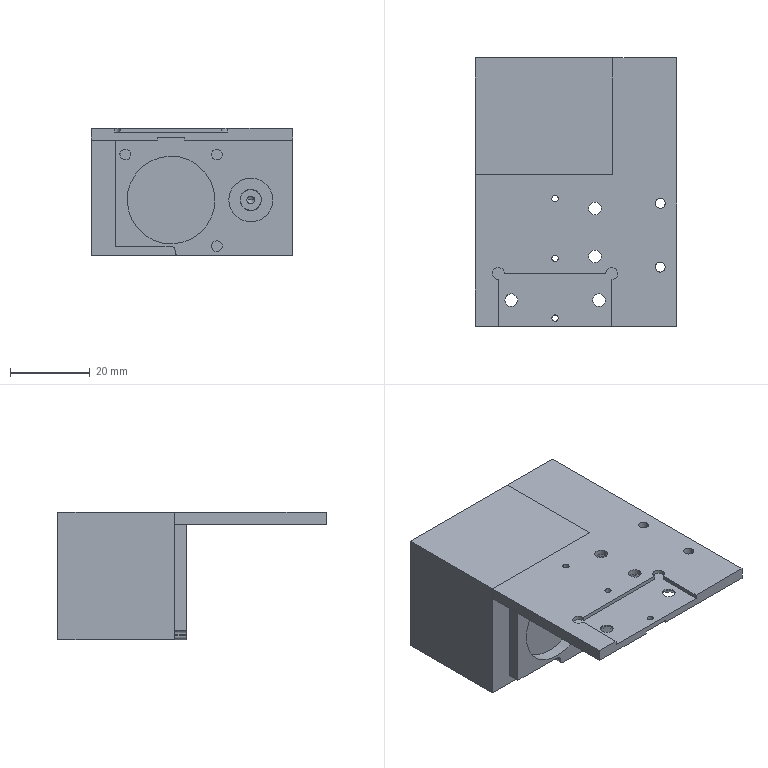NC program | NX | posted with a generic post | part box 50.5 x 67.3 x 32 mm
Whole program:
N10 G17 G21 G94 G90
(ZLEVEL_PROFILE , TOOL : D10)
N12 T10 M6
N14 G54
N16 G17 G0 G90 X35.272 Y-32.059 B0. C0. S9500 M3
N18 G43 Z30. H10
N20 Z-14.5
N22 G94 G1 Z-16. F1500.
N24 X34.516 Y-30.75
N26 G3 X33.65 Y-30.25 R1.
N28 G1 X-33.65
N30 G2 X-38.65 Y-25.25 R5.
N32 G1 Y25.25
N34 G2 X-33.65 Y30.25 R5.
N36 G1 X33.65
N38 G2 X38.65 Y25.25 R5.
N40 G1 Y-25.25
N42 G2 X33.65 Y-30.25 R5.
N44 G3 X32.784 Y-30.75 R1.
N46 G1 X31.918 Y-32.25
N48 Z-14.5
N50 G0 Z30.
N52 X35.272 Y-32.059
N54 Z-30.5
N56 G1 Z-32.
N58 X34.516 Y-30.75
N60 G3 X33.65 Y-30.25 R1.
N62 G1 X-33.65
N64 G2 X-38.65 Y-25.25 R5.
N66 G1 Y25.25
N68 G2 X-33.65 Y30.25 R5.
N70 G1 X33.65
N72 G2 X38.65 Y25.25 R5.
N74 G1 Y-25.25
N76 G2 X33.65 Y-30.25 R5.
N78 G3 X32.784 Y-30.75 R1.
N80 G1 X31.918 Y-32.25
N82 Z-30.5
N84 G0 Z30.
N86 M5
(FLOOR_WALL_1_COPY_1 , TOOL : D4)
N88 T04 M6
N90 G54
N92 G17 G0 G90 X36.65 Y-4.442 B0. C0. S9500 M3
N94 G43 Z30. H4
N96 Z-0.3
N98 G94 G1 X35.85 Y-4.904 F1000.
N100 G3 X35.65 Y-5.25 R0.4
N102 G1 Y-17.35 F2500.
N104 X22.55
N106 Y6.85
N108 X35.65
N110 Y-5.25
N112 X33.65
N114 Y-15.35
N116 X24.55
N118 Y4.85
N120 X33.65
N122 Y-5.25
N124 X31.65
N126 Y-13.35
N128 X26.55
N130 Y2.85
N132 X31.65
N134 Y-5.25
N136 X29.65
N138 Y-11.35
N140 X28.55
N142 Y0.85
N144 X29.65
N146 Y-5.25
N148 G3 X29.85 Y-5.596 R0.4
N150 G0 Z30.
N152 X36.65 Y-4.442
N154 Z-0.6
N156 G1 X35.85 Y-4.904 F1000.
N158 G3 X35.65 Y-5.25 R0.4
N160 G1 Y-17.35 F2500.
N162 X22.55
N164 Y6.85
N166 X35.65
N168 Y-5.25
N170 X33.65
N172 Y-15.35
N174 X24.55
N176 Y4.85
N178 X33.65
N180 Y-5.25
N182 X31.65
N184 Y-13.35
N186 X26.55
N188 Y2.85
N190 X31.65
N192 Y-5.25
N194 X29.65
N196 Y-11.35
N198 X28.55
N200 Y0.85
N202 X29.65
N204 Y-5.25
N206 G3 X29.85 Y-5.596 R0.4
N208 G0 Z30.
N210 X36.65 Y-4.442
N212 Z-0.9
N214 G1 X35.85 Y-4.904 F1000.
N216 G3 X35.65 Y-5.25 R0.4
N218 G1 Y-17.35 F2500.
N220 X22.55
N222 Y6.85
N224 X35.65
N226 Y-5.25
N228 X33.65
N230 Y-15.35
N232 X24.55
N234 Y4.85
N236 X33.65
N238 Y-5.25
N240 X31.65
N242 Y-13.35
N244 X26.55
N246 Y2.85
N248 X31.65
N250 Y-5.25
N252 X29.65
N254 Y-11.35
N256 X28.55
N258 Y0.85
N260 X29.65
N262 Y-5.25
N264 G3 X29.85 Y-5.596 R0.4
N266 G0 Z30.
(FLOOR_WALL_1_COPY , TOOL : D4)
N268 X36.65 Y6.404
N270 Z0.
N272 G1 Z-1. F1000.
N274 X35.45
N276 G3 X35.65 Y6.75 R0.4
N278 G1 Y-17.25 F1500.
N280 X33.793
N282 Y6.75
N284 X31.936
N286 Y-17.25
N288 X30.079
N290 Y6.75
N292 X28.221
N294 Y-17.25
N296 X26.364
N298 Y6.75
N300 X24.507
N302 Y-17.25
N304 X22.65
N306 Y6.75
N308 Z0.
N310 G0 Z5.5
N312 X36.65 Y5.618
N314 Z0.
N316 G1 Z-1. F1000.
N318 X35.996 Y6.75
N320 G3 X35.65 Y6.95 R0.4
N322 G1 X22.45 F1500.
N324 Y-17.45
N326 X35.65
N328 G3 X35.996 Y-17.25 R0.4
N330 G1 X36.65 Y-16.118
N332 Z0.
N334 G0 Z30.
N336 M5
N338 M2